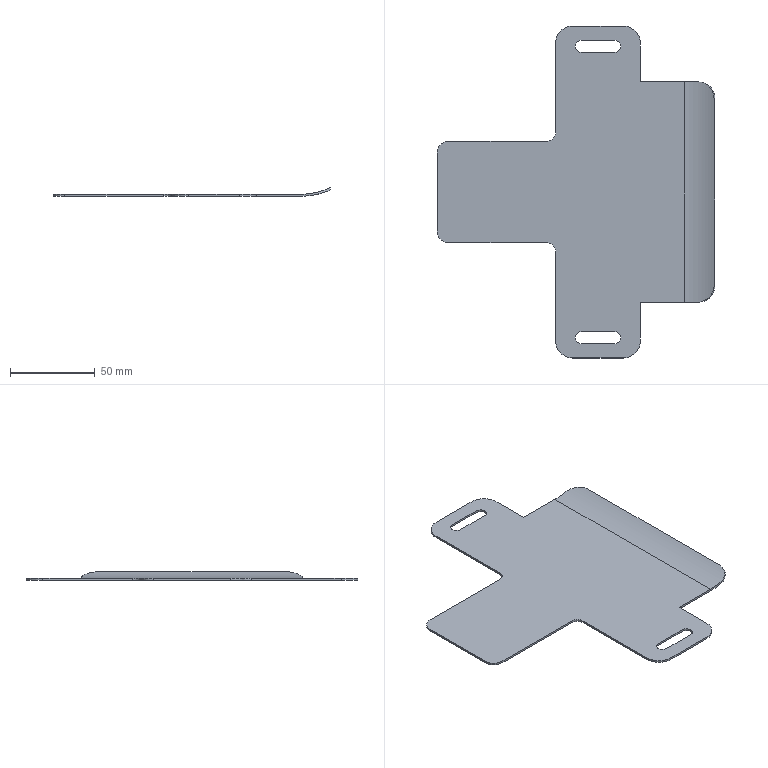Part | STEP file | YBQDJ-YB-34 | 1 solid | 34 faces | box 164.076 x 196 x 5.026 mm | volume 23129 mm3 | plane 18 | cylinder 16 | commonest cylinder face diameters 20 x6 7 x4 10 x2 14 x2 83.301 x1 85.701 x1